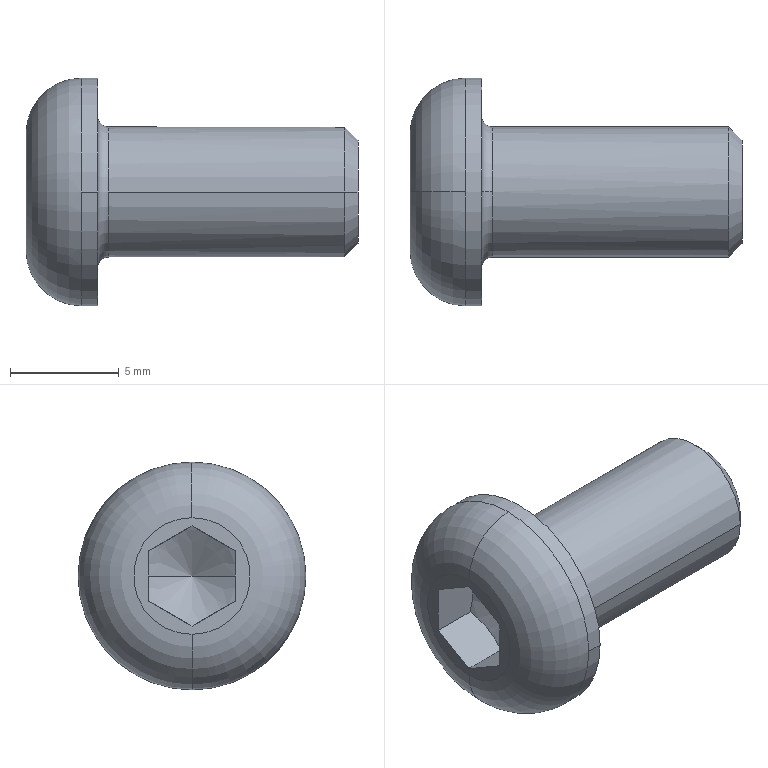Part | STEP file | ISO 7380-1 - M6 x 12 | 1 solid | 21 faces | box 15.3 x 10.5 x 10.5 mm | volume 545.38 mm3 | plane 9 | torus 4 | cylinder 4 | cone 4 | commonest cylinder face diameters 6 x2 10.5 x2